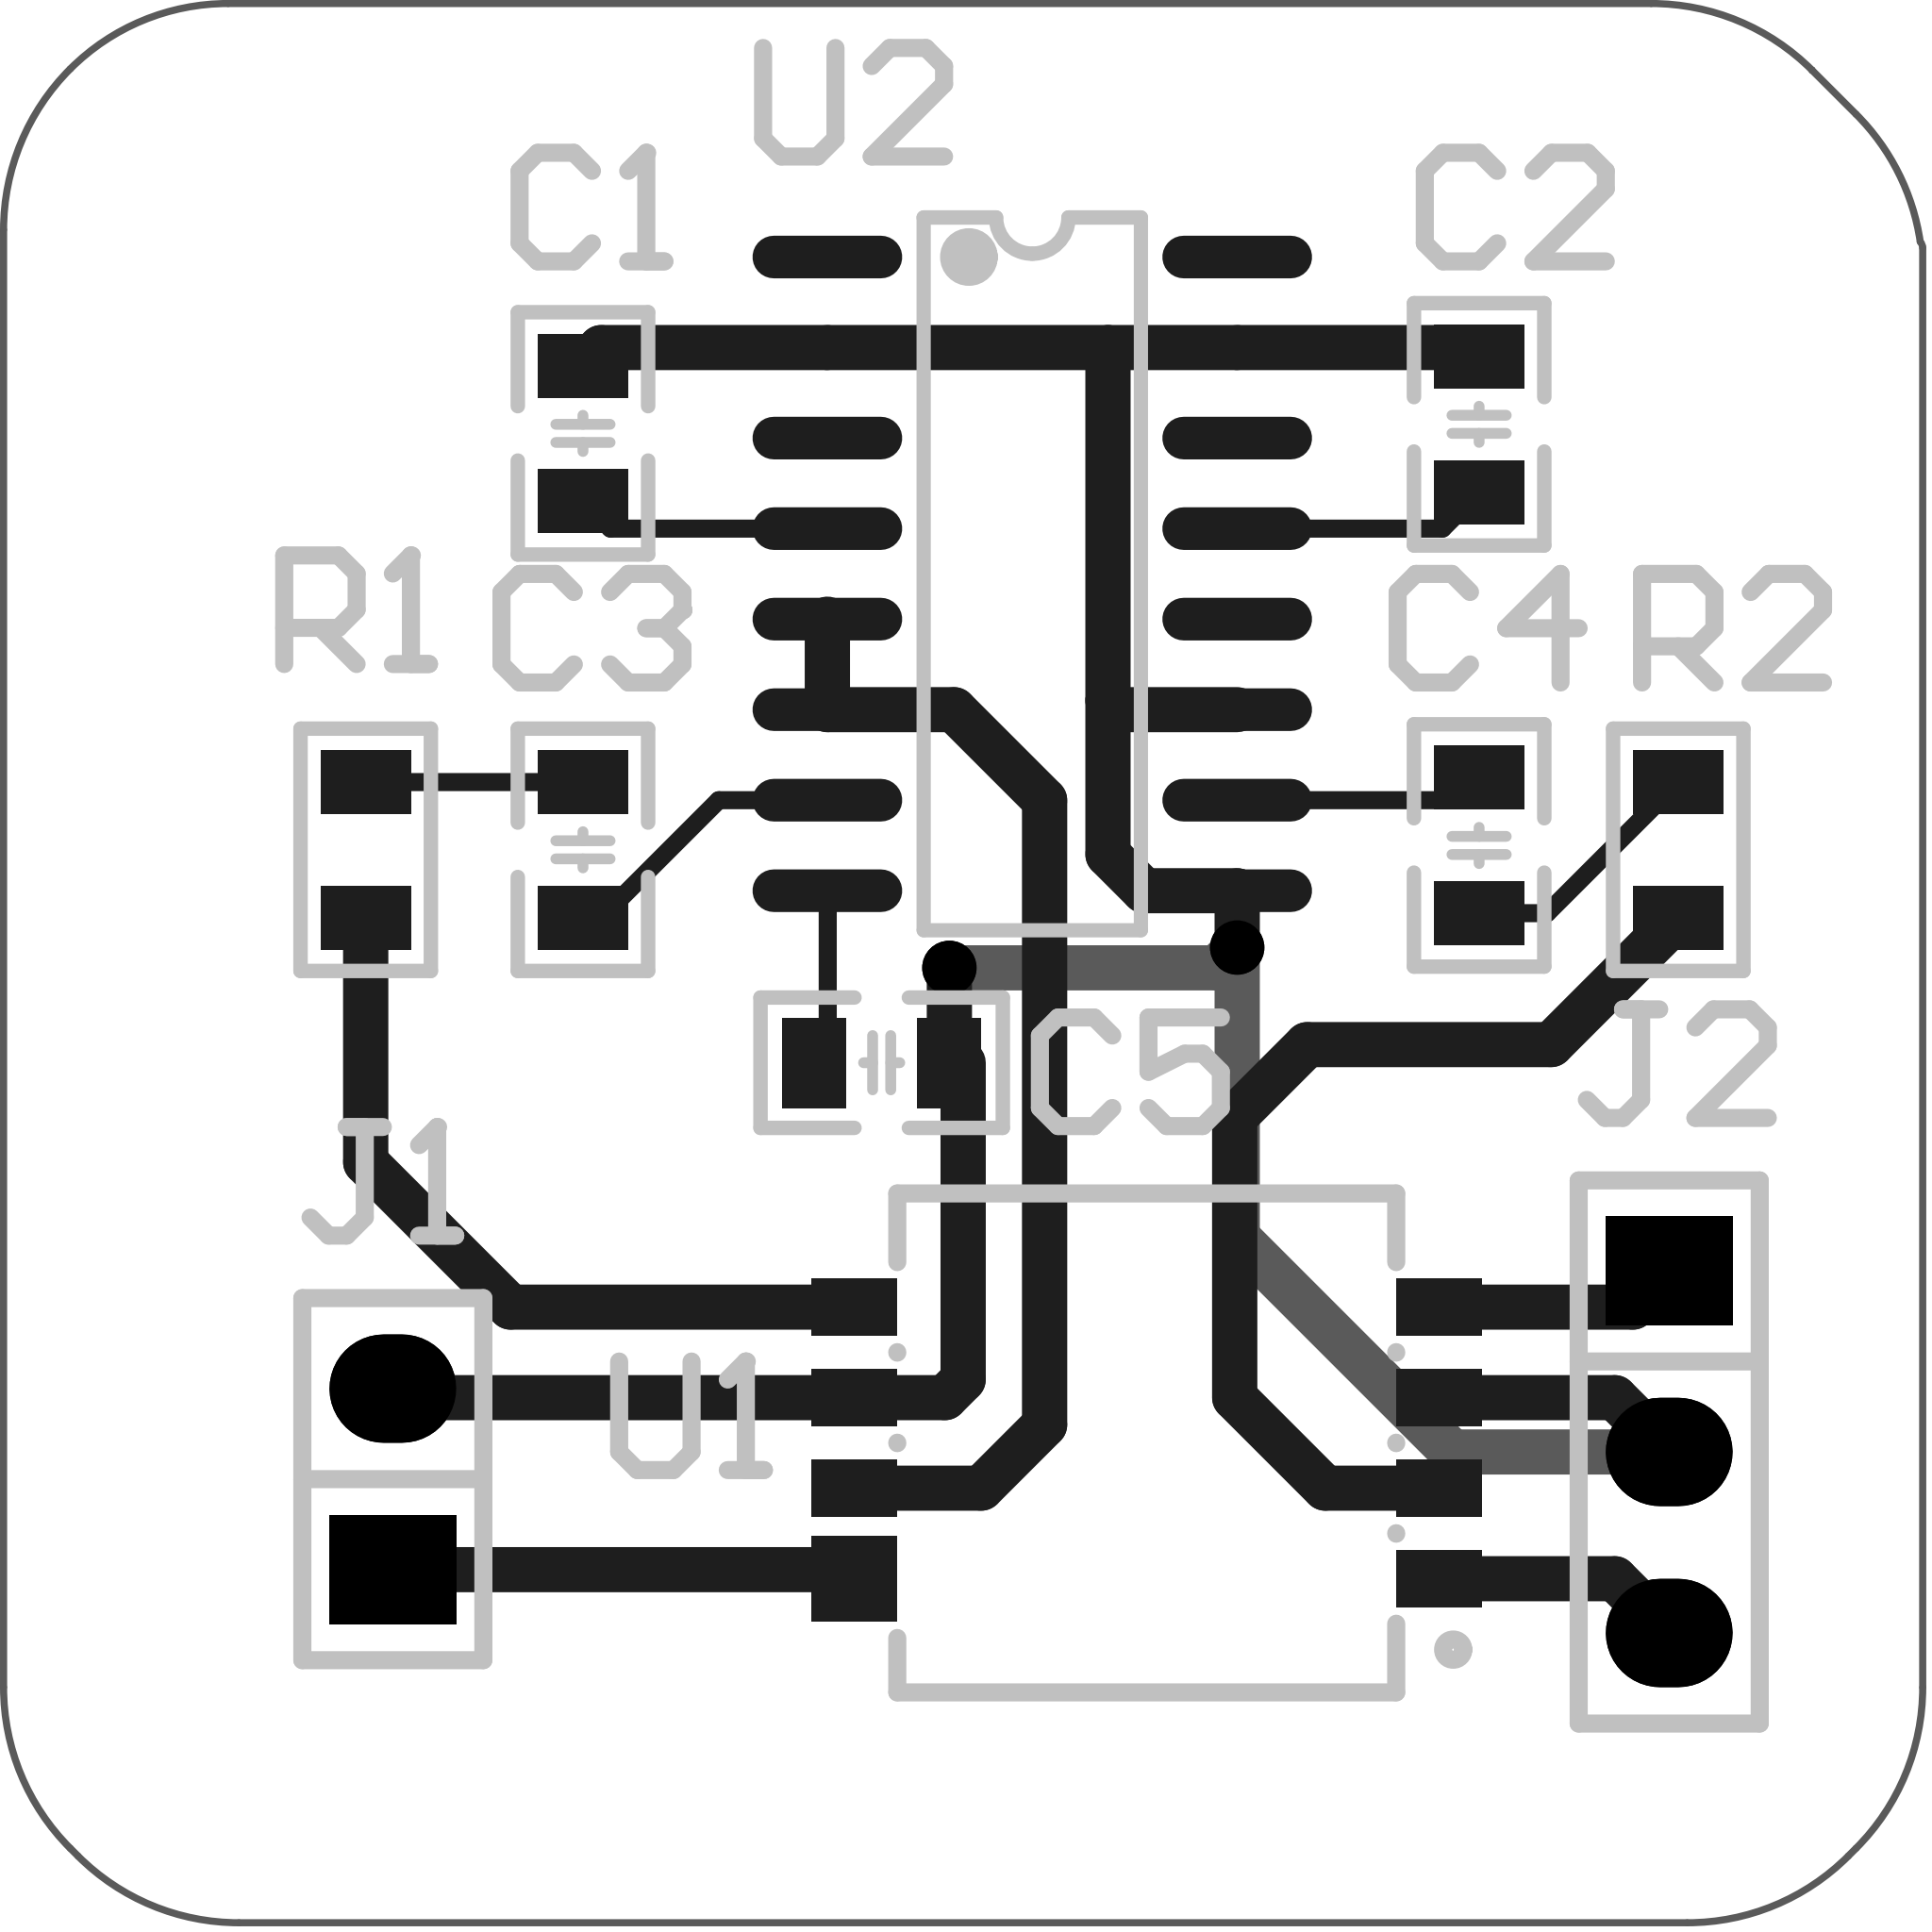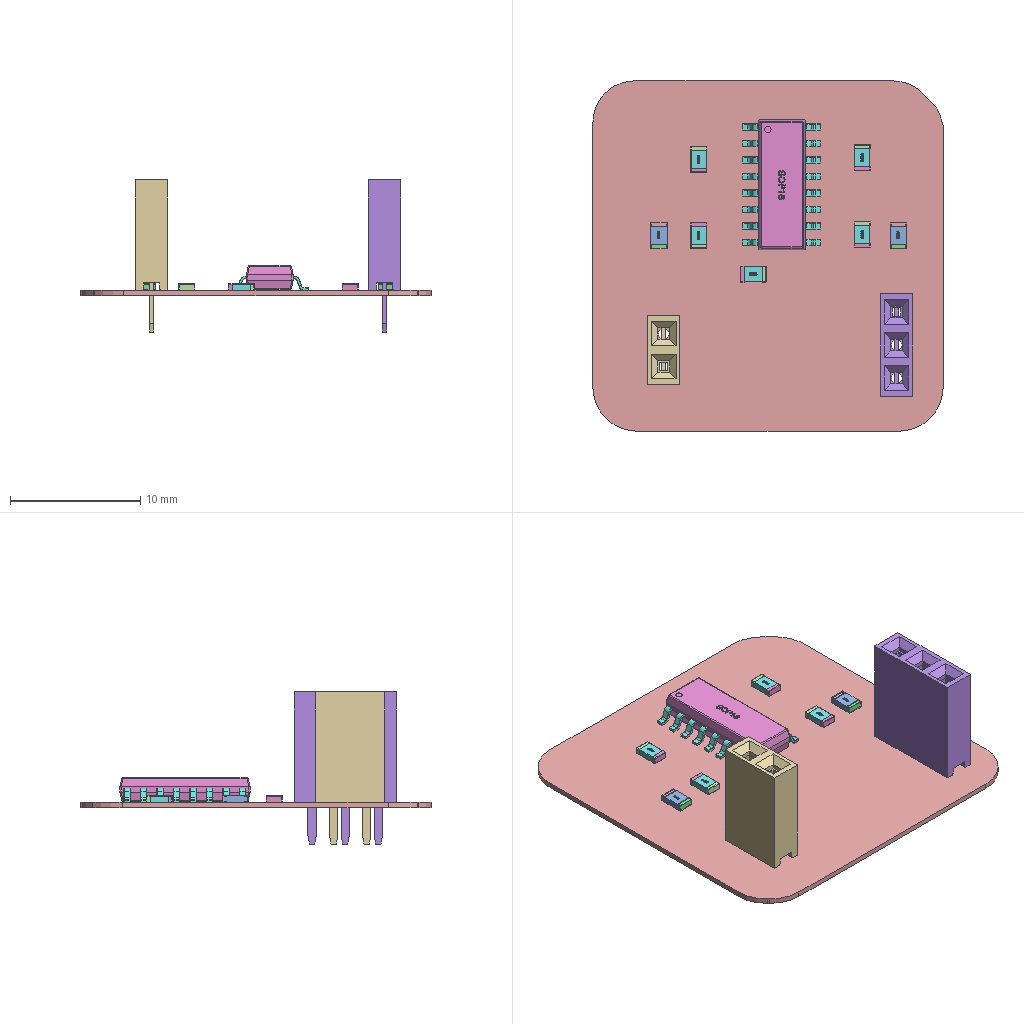Circuit board layout | Altium Designer | box 26.9 x 26.9 x 11.7 mm
Layer stack:
# Altium Designer layer stack of  (unit mm; dielectric type: 0 none, 1 core, 2 prepreg, 3 surface material)
index,name,kind,layer,copper_thickness_mm,dielectric_type,dielectric_thickness_mm,dielectric_material,dielectric_constant
0,Top Paste,other,,,,,,
1,Top Overlay,other,,,,,,
2,Top Solder,dielectric,,,3,0.0102,Solder Resist,3.5
3,Top Layer,copper,Top Layer,0.0356,,,,
4,Dielectric 1,dielectric,,,0,0.32,FR-4,4.8
5,Bottom Layer,copper,Bottom Layer,0.0356,,,,
6,Bottom Solder,dielectric,,,3,0.0102,Solder Resist,3.5
7,Bottom Overlay,other,,,,,,
8,Bottom Paste,other,,,,,,
# drill layer pairs: low layer,high layer
drill_pair,Top Layer,Bottom Layer
Part placement:
Designator,Comment,Layer,Footprint,Center-X(mm),Center-Y(mm),Rotation
C1,104,TopLayer,C_0805_L,87.376,67.122,270
C2,104,TopLayer,C_0805_L,99.949,67.249,270
C3,104,TopLayer,C_0805_L,87.376,61.28,90
C4,104,TopLayer,C_0805_L,99.949,61.341,270
C5,104,TopLayer,C_0805_L,91.567,58.293,180
J1,Female HDR1X2,TopLayer,Fe-HDR1X2/2.54-S,84.709,52.451,90
J2,Female HDR1X3,TopLayer,Fe-HDR1X3/2.54-S,102.616,52.832,0
R1,103,TopLayer,R_0805_L,84.328,61.28,90
R2,103,TopLayer,R_0805_L,102.743,61.28,90
U1,A50K,TopLayer,SOP-8_L7.0-W7.0-P1.27-LS8.6-BL,95.286,52.959,90
U2,PAM8406,TopLayer,SOP16,93.68,65.151,0
Pad and via stacks:
# Altium Designer via and pad stacks of  (unit mm). Each distinct definition once, with the count of objects using it.
# via: kind,start_layer,end_layer,hole_mm,diameter_mm,mode(0 simple;1 top-mid-bottom;2 full stack),diameter_per_layer,count,example_net
# pad: kind,layer,hole_mm,hole_type(0 round;1 square;2 slot),plating,top_size,top_shape(1 round;2 rect;3 octagon;9 rounded rect),mid_size,bottom_size,mode,footprint,size_per_layer,count,example
pad,Top Layer,0,0,plated,1.27x0.889,2,1.27x0.889,1.27x0.889,0,C 0805_L,,10,C5.2
pad,Top Layer,0,0,plated,1.27x0.889,2,1.27x0.889,1.27x0.889,0,R 0805_L,,4,R2.2
pad,Top Layer,0,0,plated,0.6x2.1,1,0.6x2.1,0.6x2.1,0,SOP16,,16,U2.9
pad,Top Layer,0,0,plated,0.8x1.2,2,0.8x1.2,0.8x1.2,0,SOP-8_L7.0-W7.0-P1.27-LS8.6-BL,,7,U1.1
pad,Top Layer,0,0,plated,1.2x1.2,2,1.2x1.2,1.2x1.2,0,SOP-8_L7.0-W7.0-P1.27-LS8.6-BL,,1,U1.8
pad,Multi-Layer,0.8128,0,plated,1.524x1.778,1,1.524x1.778,1.524x1.778,0,Fe-HDR1X3/2.54-S,,2,J2.3
pad,Multi-Layer,0.8128,0,plated,1.524x1.778,2,1.524x1.778,1.524x1.778,0,Fe-HDR1X3/2.54-S,,1,J2.1
pad,Multi-Layer,0.8128,0,plated,1.524x1.778,1,1.524x1.778,1.524x1.778,0,Fe-HDR1X2/2.54-S,,1,J1.2
pad,Multi-Layer,0.8128,0,plated,1.524x1.778,2,1.524x1.778,1.524x1.778,0,Fe-HDR1X2/2.54-S,,1,J1.1
via,Top Layer,Bottom Layer,0.381,0.762,0,,2,GND
Design rules, without the lines most boards share:
# Altium Designer design rules of  (exported by Altium Designer, unit mm)
# columns: name | kind | enabled | priority | scope1 | scope2 | descriptor | typed fields (field=value)
SilkToSilkClearance | 55 | enabled | 1 | All | All | Silk to Silk (Clearance=0mil) (All),(All) |
SilkToSolderMaskClearance | 54 | enabled | 1 | IsPad | All | Silk To Solder Mask (Clearance=0mil) (IsPad),(All) |
MinimumSolderMaskSliver | 53 | enabled | 1 | All | All | Minimum Solder Mask Sliver (Gap=0mil) (All),(All) |
HoleToHoleClearance | 52 | enabled | 1 | All | All | Hole To Hole Clearance (Gap=10mil) (All),(All) | gap=0.254
DiffPairsRouting | 51 | enabled | 1 | All | All | Differential Pairs Uncoupled Length using the Gap Constraints (Min=10mil) (Max=10mil) (Prefered=10mil)  and Width Constraints (Min=15mil) (Max=15mil) (Prefered=15mil) (All) |
SolderMaskExpansion | 13 | enabled | 1 | All | All | Solder Mask Expansion (Expansion =4mil) (All) | expansion=0.1016
PasteMaskExpansion | 14 | enabled | 1 | All | All | Paste Mask Expansion (Expansion =0mil) (All) | expansion=0
RoutingVias | 11 | enabled | 1 | All | All | Routing Via (MinHoleWidth=28mil) (MaxHoleWidth=28mil) (PreferredHoleWidth=28mil) (MinWidth=50mil) (MaxWidth=50mil) (PreferedWidth=50mil) (All) | via_min_hole=0.7112 via_max_hole=0.7112 via_preferred_diameter=1.27 via_preferred_hole=0.7112
Width | 2 | enabled | 1 | All | All | Width Constraint (Min=10mil) (Max=30mil) (Preferred=10mil) (All) |
PolygonConnect | 20 | enabled | 1 | All | All | Polygon Connect Rule(Relief Connect )(Conductor Width=10mil) (Relief Angle=90 Angle) (Entries=4) (Air Gap Width=10mil) (All),(All) | connect_style(0=relief,1=direct,2=none)=0 relief_conductor_width=0.254 relief_entries=4
PlaneConnect | 6 | enabled | 1 | All | All | Power Plane Connect Rule(Relief Connect )(Expansion=20mil) (Conductor Width=10mil) (Air Gap=10mil) (Entries=4) (All) | relief_conductor_width=0.254 relief_entries=4 relief_expansion=0.508
Clearance | 0 | enabled | 1 | All | All | Clearance Constraint (Gap=10mil) (All),(All) | gap=0.254
Classes set for this board:
# Altium Designer classes of  (member kind: 0 net, 1 component, 2 from-to, 3 pad, 4 layer, 5 differential pair, 6 design channel, 7 polygon, 8 structure, 9 xSignal)
# columns: class name | member kind | superclass | members
Sheet1 | 1 | no | C1; C2; C3; C4; C5; J1; J2; R1; R2; U1; U2;